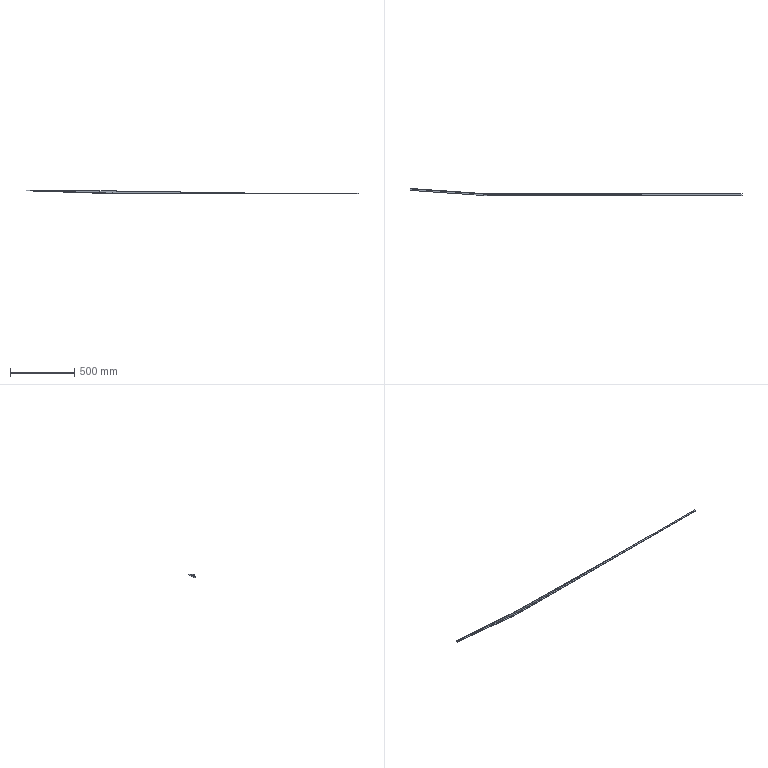Part | SolidWorks | features BaseBody 1 | 1 solid | 20 faces | box 2576 x 54.755 x 25.641 mm | volume 177267 mm3 | plane 20
STEP:
#1=CARTESIAN_POINT('',(-2.164,63.36,25.883));
#2=VERTEX_POINT('',#1);
#3=CARTESIAN_POINT('',(97.633,63.419,22.713));
#4=VERTEX_POINT('',#3);
#5=CARTESIAN_POINT('',(-2.164,63.36,25.883));
#6=CARTESIAN_POINT('',(31.101,63.38,24.826));
#7=CARTESIAN_POINT('',(64.367,63.4,23.77));
#8=CARTESIAN_POINT('',(97.633,63.419,22.713));
#9=B_SPLINE_CURVE_WITH_KNOTS('',3,(#5,#6,#7,#8),.UNSPECIFIED.,.F.,.F.,(4,4),(0.,1.),.UNSPECIFIED.);
#10=EDGE_CURVE('',#2,#4,#9,.T.);
#11=ORIENTED_EDGE('',*,*,#10,.F.);
#12=CARTESIAN_POINT('',(-2.388,60.16,25.827));
#13=VERTEX_POINT('',#12);
#14=CARTESIAN_POINT('',(-2.388,60.16,25.827));
#15=CARTESIAN_POINT('',(-2.313,61.227,25.845));
#16=CARTESIAN_POINT('',(-2.239,62.293,25.864));
#17=CARTESIAN_POINT('',(-2.164,63.36,25.883));
#18=B_SPLINE_CURVE_WITH_KNOTS('',3,(#14,#15,#16,#17),.UNSPECIFIED.,.F.,.F.,(4,4),(0.,1.),.UNSPECIFIED.);
#19=EDGE_CURVE('',#13,#2,#18,.T.);
#20=ORIENTED_EDGE('',*,*,#19,.F.);
#21=CARTESIAN_POINT('',(97.633,60.22,22.65));
#22=VERTEX_POINT('',#21);
#23=CARTESIAN_POINT('',(97.633,60.22,22.65));
#24=CARTESIAN_POINT('',(64.293,60.2,23.709));
#25=CARTESIAN_POINT('',(30.952,60.18,24.768));
#26=CARTESIAN_POINT('',(-2.388,60.16,25.827));
#27=B_SPLINE_CURVE_WITH_KNOTS('',3,(#23,#24,#25,#26),.UNSPECIFIED.,.F.,.F.,(4,4),(0.,1.),.UNSPECIFIED.);
#28=EDGE_CURVE('',#22,#13,#27,.T.);
#29=ORIENTED_EDGE('',*,*,#28,.F.);
#30=CARTESIAN_POINT('',(97.633,63.419,22.713));
#31=CARTESIAN_POINT('',(97.633,62.353,22.692));
#32=CARTESIAN_POINT('',(97.633,61.287,22.671));
#33=CARTESIAN_POINT('',(97.633,60.22,22.65));
#34=B_SPLINE_CURVE_WITH_KNOTS('',3,(#30,#31,#32,#33),.UNSPECIFIED.,.F.,.F.,(4,4),(0.,1.),.UNSPECIFIED.);
#35=EDGE_CURVE('',#4,#22,#34,.T.);
#36=ORIENTED_EDGE('',*,*,#35,.F.);
#37=EDGE_LOOP('',(#11,#20,#29,#36));
#38=FACE_OUTER_BOUND('',#37,.T.);
#39=CARTESIAN_POINT('',(98.233,60.141,22.63));
#40=DIRECTION('',(-0.03175,0.01966,-0.9993));
#41=DIRECTION('',(-0.9995,0.,0.03175));
#42=AXIS2_PLACEMENT_3D('',#39,#40,#41);
#43=PLANE('',#42);
#44=ADVANCED_FACE('',(#38),#43,.F.);
#45=ORIENTED_EDGE('',*,*,#35,.T.);
#46=CARTESIAN_POINT('',(1223.741,60.566,5.051));
#47=VERTEX_POINT('',#46);
#48=CARTESIAN_POINT('',(660.687,60.393,13.851));
#49=DIRECTION('',(-0.9999,-0.0003075,0.01563));
#50=VECTOR('',#49,1000.);
#51=LINE('',#48,#50);
#52=EDGE_CURVE('',#47,#22,#51,.T.);
#53=ORIENTED_EDGE('',*,*,#52,.F.);
#54=CARTESIAN_POINT('',(1223.741,63.766,5.114));
#55=VERTEX_POINT('',#54);
#56=CARTESIAN_POINT('',(1223.741,62.166,5.082));
#57=DIRECTION('',(0.,-0.9998,-0.01967));
#58=VECTOR('',#57,1000.);
#59=LINE('',#56,#58);
#60=EDGE_CURVE('',#55,#47,#59,.T.);
#61=ORIENTED_EDGE('',*,*,#60,.F.);
#62=CARTESIAN_POINT('',(660.687,63.593,13.914));
#63=DIRECTION('',(0.9999,0.0003075,-0.01563));
#64=VECTOR('',#63,1000.);
#65=LINE('',#62,#64);
#66=EDGE_CURVE('',#4,#55,#65,.T.);
#67=ORIENTED_EDGE('',*,*,#66,.F.);
#68=EDGE_LOOP('',(#45,#53,#61,#67));
#69=FACE_OUTER_BOUND('',#68,.T.);
#70=CARTESIAN_POINT('',(97.633,60.22,22.65));
#71=DIRECTION('',(-0.01563,0.01967,-0.9997));
#72=DIRECTION('',(0.,0.9998,0.01967));
#73=AXIS2_PLACEMENT_3D('',#70,#71,#72);
#74=PLANE('',#73);
#75=ADVANCED_FACE('',(#69),#74,.F.);
#76=CARTESIAN_POINT('',(-2.276,63.36,25.883));
#77=VERTEX_POINT('',#76);
#78=CARTESIAN_POINT('',(-2.164,63.36,25.883));
#79=CARTESIAN_POINT('',(-2.202,63.36,25.883));
#80=CARTESIAN_POINT('',(-2.239,63.36,25.883));
#81=CARTESIAN_POINT('',(-2.276,63.36,25.883));
#82=B_SPLINE_CURVE_WITH_KNOTS('',3,(#78,#79,#80,#81),.UNSPECIFIED.,.F.,.F.,(4,4),(0.,1.),.UNSPECIFIED.);
#83=EDGE_CURVE('',#2,#77,#82,.T.);
#84=ORIENTED_EDGE('',*,*,#83,.F.);
#85=ORIENTED_EDGE('',*,*,#10,.T.);
#86=CARTESIAN_POINT('',(97.303,63.829,1.914));
#87=VERTEX_POINT('',#86);
#88=CARTESIAN_POINT('',(97.303,63.829,1.914));
#89=CARTESIAN_POINT('',(97.413,63.692,8.847));
#90=CARTESIAN_POINT('',(97.523,63.556,15.78));
#91=CARTESIAN_POINT('',(97.633,63.419,22.713));
#92=B_SPLINE_CURVE_WITH_KNOTS('',3,(#88,#89,#90,#91),.UNSPECIFIED.,.F.,.F.,(4,4),(0.,1.),.UNSPECIFIED.);
#93=EDGE_CURVE('',#87,#4,#92,.T.);
#94=ORIENTED_EDGE('',*,*,#93,.F.);
#95=CARTESIAN_POINT('',(-2.937,63.769,5.098));
#96=VERTEX_POINT('',#95);
#97=CARTESIAN_POINT('',(-2.937,63.769,5.098));
#98=CARTESIAN_POINT('',(30.476,63.789,4.036));
#99=CARTESIAN_POINT('',(63.889,63.809,2.975));
#100=CARTESIAN_POINT('',(97.303,63.829,1.914));
#101=B_SPLINE_CURVE_WITH_KNOTS('',3,(#97,#98,#99,#100),.UNSPECIFIED.,.F.,.F.,(4,4),(0.,1.),.UNSPECIFIED.);
#102=EDGE_CURVE('',#96,#87,#101,.T.);
#103=ORIENTED_EDGE('',*,*,#102,.F.);
#104=CARTESIAN_POINT('',(-2.276,63.36,25.883));
#105=CARTESIAN_POINT('',(-2.496,63.496,18.954));
#106=CARTESIAN_POINT('',(-2.717,63.632,12.026));
#107=CARTESIAN_POINT('',(-2.937,63.769,5.098));
#108=B_SPLINE_CURVE_WITH_KNOTS('',3,(#104,#105,#106,#107),.UNSPECIFIED.,.F.,.F.,(4,4),(0.,1.),.UNSPECIFIED.);
#109=EDGE_CURVE('',#77,#96,#108,.T.);
#110=ORIENTED_EDGE('',*,*,#109,.F.);
#111=EDGE_LOOP('',(#84,#85,#94,#103,#110));
#112=FACE_OUTER_BOUND('',#111,.T.);
#113=CARTESIAN_POINT('',(-2.937,63.36,25.883));
#114=DIRECTION('',(-0.0000264,-0.9998,-0.01967));
#115=DIRECTION('',(0.,0.01967,-0.9998));
#116=AXIS2_PLACEMENT_3D('',#113,#114,#115);
#117=PLANE('',#116);
#118=ADVANCED_FACE('',(#112),#117,.F.);
#119=CARTESIAN_POINT('',(-575.334,100.207,27.204));
#120=VERTEX_POINT('',#119);
#121=CARTESIAN_POINT('',(-575.111,103.398,27.26));
#122=VERTEX_POINT('',#121);
#123=CARTESIAN_POINT('',(-575.334,100.207,27.204));
#124=CARTESIAN_POINT('',(-575.26,101.27,27.223));
#125=CARTESIAN_POINT('',(-575.185,102.334,27.241));
#126=CARTESIAN_POINT('',(-575.111,103.398,27.26));
#127=B_SPLINE_CURVE_WITH_KNOTS('',3,(#123,#124,#125,#126),.UNSPECIFIED.,.F.,.F.,(4,4),(0.,1.),.UNSPECIFIED.);
#128=EDGE_CURVE('',#120,#122,#127,.T.);
#129=ORIENTED_EDGE('',*,*,#128,.F.);
#130=CARTESIAN_POINT('',(-2.388,60.16,25.827));
#131=CARTESIAN_POINT('',(-193.37,73.509,26.286));
#132=CARTESIAN_POINT('',(-384.352,86.858,26.745));
#133=CARTESIAN_POINT('',(-575.334,100.207,27.204));
#134=B_SPLINE_CURVE_WITH_KNOTS('',3,(#130,#131,#132,#133),.UNSPECIFIED.,.F.,.F.,(4,4),(0.,1.),.UNSPECIFIED.);
#135=EDGE_CURVE('',#13,#120,#134,.T.);
#136=ORIENTED_EDGE('',*,*,#135,.F.);
#137=ORIENTED_EDGE('',*,*,#19,.T.);
#138=ORIENTED_EDGE('',*,*,#83,.T.);
#139=CARTESIAN_POINT('',(-575.111,103.398,27.26));
#140=CARTESIAN_POINT('',(-384.166,90.052,26.801));
#141=CARTESIAN_POINT('',(-193.221,76.706,26.342));
#142=CARTESIAN_POINT('',(-2.276,63.36,25.883));
#143=B_SPLINE_CURVE_WITH_KNOTS('',3,(#139,#140,#141,#142),.UNSPECIFIED.,.F.,.F.,(4,4),(0.,1.),.UNSPECIFIED.);
#144=EDGE_CURVE('',#122,#77,#143,.T.);
#145=ORIENTED_EDGE('',*,*,#144,.F.);
#146=EDGE_LOOP('',(#129,#136,#137,#138,#145));
#147=FACE_OUTER_BOUND('',#146,.T.);
#148=CARTESIAN_POINT('',(-575.334,60.148,26.502));
#149=DIRECTION('',(-0.001178,0.01753,-0.9998));
#150=DIRECTION('',(0.,0.9998,0.01753));
#151=AXIS2_PLACEMENT_3D('',#148,#149,#150);
#152=PLANE('',#151);
#153=ADVANCED_FACE('',(#147),#152,.F.);
#154=ORIENTED_EDGE('',*,*,#28,.T.);
#155=CARTESIAN_POINT('',(-2.947,60.506,8.236));
#156=VERTEX_POINT('',#155);
#157=CARTESIAN_POINT('',(-2.947,60.506,8.236));
#158=CARTESIAN_POINT('',(-2.761,60.391,14.1));
#159=CARTESIAN_POINT('',(-2.574,60.276,19.963));
#160=CARTESIAN_POINT('',(-2.388,60.16,25.827));
#161=B_SPLINE_CURVE_WITH_KNOTS('',3,(#157,#158,#159,#160),.UNSPECIFIED.,.F.,.F.,(4,4),(0.,1.),.UNSPECIFIED.);
#162=EDGE_CURVE('',#156,#13,#161,.T.);
#163=ORIENTED_EDGE('',*,*,#162,.F.);
#164=CARTESIAN_POINT('',(97.353,60.566,5.051));
#165=VERTEX_POINT('',#164);
#166=CARTESIAN_POINT('',(97.353,60.566,5.051));
#167=CARTESIAN_POINT('',(63.92,60.546,6.112));
#168=CARTESIAN_POINT('',(30.486,60.526,7.174));
#169=CARTESIAN_POINT('',(-2.947,60.506,8.236));
#170=B_SPLINE_CURVE_WITH_KNOTS('',3,(#166,#167,#168,#169),.UNSPECIFIED.,.F.,.F.,(4,4),(0.,1.),.UNSPECIFIED.);
#171=EDGE_CURVE('',#165,#156,#170,.T.);
#172=ORIENTED_EDGE('',*,*,#171,.F.);
#173=CARTESIAN_POINT('',(97.633,60.22,22.65));
#174=CARTESIAN_POINT('',(97.54,60.336,16.784));
#175=CARTESIAN_POINT('',(97.447,60.451,10.917));
#176=CARTESIAN_POINT('',(97.353,60.566,5.051));
#177=B_SPLINE_CURVE_WITH_KNOTS('',3,(#173,#174,#175,#176),.UNSPECIFIED.,.F.,.F.,(4,4),(0.,1.),.UNSPECIFIED.);
#178=EDGE_CURVE('',#22,#165,#177,.T.);
#179=ORIENTED_EDGE('',*,*,#178,.F.);
#180=EDGE_LOOP('',(#154,#163,#172,#179));
#181=FACE_OUTER_BOUND('',#180,.T.);
#182=CARTESIAN_POINT('',(-3.55,60.572,4.926));
#183=DIRECTION('',(0.0000264,0.9998,0.01967));
#184=DIRECTION('',(0.,-0.01967,0.9998));
#185=AXIS2_PLACEMENT_3D('',#182,#183,#184);
#186=PLANE('',#185);
#187=ADVANCED_FACE('',(#181),#186,.F.);
#188=ORIENTED_EDGE('',*,*,#93,.T.);
#189=ORIENTED_EDGE('',*,*,#66,.T.);
#190=CARTESIAN_POINT('',(2000.,63.766,5.114));
#191=VERTEX_POINT('',#190);
#192=CARTESIAN_POINT('',(1048.651,63.766,5.114));
#193=DIRECTION('',(1.,0.,0.));
#194=VECTOR('',#193,1000.);
#195=LINE('',#192,#194);
#196=EDGE_CURVE('',#55,#191,#195,.T.);
#197=ORIENTED_EDGE('',*,*,#196,.T.);
#198=CARTESIAN_POINT('',(2000.,63.829,1.914));
#199=VERTEX_POINT('',#198);
#200=CARTESIAN_POINT('',(2000.,63.624,12.314));
#201=DIRECTION('',(0.,0.01967,-0.9998));
#202=VECTOR('',#201,1000.);
#203=LINE('',#200,#202);
#204=EDGE_CURVE('',#191,#199,#203,.T.);
#205=ORIENTED_EDGE('',*,*,#204,.T.);
#206=CARTESIAN_POINT('',(1048.651,63.829,1.914));
#207=DIRECTION('',(-1.,0.,0.));
#208=VECTOR('',#207,1000.);
#209=LINE('',#206,#208);
#210=EDGE_CURVE('',#199,#87,#209,.T.);
#211=ORIENTED_EDGE('',*,*,#210,.T.);
#212=EDGE_LOOP('',(#188,#189,#197,#205,#211));
#213=FACE_OUTER_BOUND('',#212,.T.);
#214=CARTESIAN_POINT('',(97.303,63.829,1.914));
#215=DIRECTION('',(0.,0.9998,0.01967));
#216=DIRECTION('',(0.,-0.01967,0.9998));
#217=AXIS2_PLACEMENT_3D('',#214,#215,#216);
#218=PLANE('',#217);
#219=ADVANCED_FACE('',(#213),#218,.T.);
#220=ORIENTED_EDGE('',*,*,#178,.T.);
#221=CARTESIAN_POINT('',(660.547,60.566,5.051));
#222=DIRECTION('',(1.,0.,0.));
#223=VECTOR('',#222,1000.);
#224=LINE('',#221,#223);
#225=EDGE_CURVE('',#165,#47,#224,.T.);
#226=ORIENTED_EDGE('',*,*,#225,.T.);
#227=ORIENTED_EDGE('',*,*,#52,.T.);
#228=EDGE_LOOP('',(#220,#226,#227));
#229=FACE_OUTER_BOUND('',#228,.T.);
#230=CARTESIAN_POINT('',(90.595,60.218,22.756));
#231=DIRECTION('',(0.,-0.9998,-0.01967));
#232=DIRECTION('',(0.,0.01967,-0.9998));
#233=AXIS2_PLACEMENT_3D('',#230,#231,#232);
#234=PLANE('',#233);
#235=ADVANCED_FACE('',(#229),#234,.T.);
#236=ORIENTED_EDGE('',*,*,#225,.F.);
#237=CARTESIAN_POINT('',(97.353,48.766,4.818));
#238=VERTEX_POINT('',#237);
#239=CARTESIAN_POINT('',(97.353,60.566,5.051));
#240=CARTESIAN_POINT('',(97.353,56.633,4.973));
#241=CARTESIAN_POINT('',(97.353,52.7,4.896));
#242=CARTESIAN_POINT('',(97.353,48.766,4.818));
#243=B_SPLINE_CURVE_WITH_KNOTS('',3,(#239,#240,#241,#242),.UNSPECIFIED.,.F.,.F.,(4,4),(0.,1.),.UNSPECIFIED.);
#244=EDGE_CURVE('',#165,#238,#243,.T.);
#245=ORIENTED_EDGE('',*,*,#244,.T.);
#246=CARTESIAN_POINT('',(2000.,48.766,4.818));
#247=VERTEX_POINT('',#246);
#248=CARTESIAN_POINT('',(1048.677,48.766,4.818));
#249=DIRECTION('',(1.,0.,0.));
#250=VECTOR('',#249,1000.);
#251=LINE('',#248,#250);
#252=EDGE_CURVE('',#238,#247,#251,.T.);
#253=ORIENTED_EDGE('',*,*,#252,.T.);
#254=CARTESIAN_POINT('',(2000.,56.266,4.966));
#255=DIRECTION('',(0.,0.9998,0.01967));
#256=VECTOR('',#255,1000.);
#257=LINE('',#254,#256);
#258=EDGE_CURVE('',#247,#191,#257,.T.);
#259=ORIENTED_EDGE('',*,*,#258,.T.);
#260=ORIENTED_EDGE('',*,*,#196,.F.);
#261=ORIENTED_EDGE('',*,*,#60,.T.);
#262=EDGE_LOOP('',(#236,#245,#253,#259,#260,#261));
#263=FACE_OUTER_BOUND('',#262,.T.);
#264=CARTESIAN_POINT('',(97.353,63.766,5.114));
#265=DIRECTION('',(0.,-0.01967,0.9998));
#266=DIRECTION('',(0.,-0.9998,-0.01967));
#267=AXIS2_PLACEMENT_3D('',#264,#265,#266);
#268=PLANE('',#267);
#269=ADVANCED_FACE('',(#263),#268,.T.);
#270=CARTESIAN_POINT('',(-575.213,103.461,24.062));
#271=VERTEX_POINT('',#270);
#272=CARTESIAN_POINT('',(-2.937,63.769,5.098));
#273=CARTESIAN_POINT('',(-193.695,77.,11.419));
#274=CARTESIAN_POINT('',(-384.454,90.23,17.741));
#275=CARTESIAN_POINT('',(-575.213,103.461,24.062));
#276=B_SPLINE_CURVE_WITH_KNOTS('',3,(#272,#273,#274,#275),.UNSPECIFIED.,.F.,.F.,(4,4),(0.,1.),.UNSPECIFIED.);
#277=EDGE_CURVE('',#96,#271,#276,.T.);
#278=ORIENTED_EDGE('',*,*,#277,.T.);
#279=CARTESIAN_POINT('',(-575.213,103.461,24.062));
#280=CARTESIAN_POINT('',(-575.179,103.44,25.128));
#281=CARTESIAN_POINT('',(-575.145,103.419,26.194));
#282=CARTESIAN_POINT('',(-575.111,103.398,27.26));
#283=B_SPLINE_CURVE_WITH_KNOTS('',3,(#279,#280,#281,#282),.UNSPECIFIED.,.F.,.F.,(4,4),(0.,1.),.UNSPECIFIED.);
#284=EDGE_CURVE('',#271,#122,#283,.T.);
#285=ORIENTED_EDGE('',*,*,#284,.T.);
#286=ORIENTED_EDGE('',*,*,#144,.T.);
#287=ORIENTED_EDGE('',*,*,#109,.T.);
#288=EDGE_LOOP('',(#278,#285,#286,#287));
#289=FACE_OUTER_BOUND('',#288,.T.);
#290=CARTESIAN_POINT('',(1.187,63.483,4.965));
#291=DIRECTION('',(0.06976,0.9974,0.01741));
#292=DIRECTION('',(-0.9976,0.06977,0.));
#293=AXIS2_PLACEMENT_3D('',#290,#291,#292);
#294=PLANE('',#293);
#295=ADVANCED_FACE('',(#289),#294,.T.);
#296=CARTESIAN_POINT('',(-3.461,48.769,4.819));
#297=VERTEX_POINT('',#296);
#298=CARTESIAN_POINT('',(97.302,48.829,1.619));
#299=VERTEX_POINT('',#298);
#300=CARTESIAN_POINT('',(-3.461,48.769,4.819));
#301=CARTESIAN_POINT('',(30.127,48.789,3.752));
#302=CARTESIAN_POINT('',(63.715,48.809,2.686));
#303=CARTESIAN_POINT('',(97.302,48.829,1.619));
#304=B_SPLINE_CURVE_WITH_KNOTS('',3,(#300,#301,#302,#303),.UNSPECIFIED.,.F.,.F.,(4,4),(0.,1.),.UNSPECIFIED.);
#305=EDGE_CURVE('',#297,#299,#304,.T.);
#306=ORIENTED_EDGE('',*,*,#305,.F.);
#307=CARTESIAN_POINT('',(-2.937,63.769,5.098));
#308=CARTESIAN_POINT('',(-3.111,58.769,5.005));
#309=CARTESIAN_POINT('',(-3.286,53.769,4.912));
#310=CARTESIAN_POINT('',(-3.461,48.769,4.819));
#311=B_SPLINE_CURVE_WITH_KNOTS('',3,(#307,#308,#309,#310),.UNSPECIFIED.,.F.,.F.,(4,4),(0.,1.),.UNSPECIFIED.);
#312=EDGE_CURVE('',#96,#297,#311,.T.);
#313=ORIENTED_EDGE('',*,*,#312,.F.);
#314=ORIENTED_EDGE('',*,*,#102,.T.);
#315=CARTESIAN_POINT('',(97.302,48.829,1.619));
#316=CARTESIAN_POINT('',(97.302,53.829,1.717));
#317=CARTESIAN_POINT('',(97.303,58.829,1.816));
#318=CARTESIAN_POINT('',(97.303,63.829,1.914));
#319=B_SPLINE_CURVE_WITH_KNOTS('',3,(#315,#316,#317,#318),.UNSPECIFIED.,.F.,.F.,(4,4),(0.,1.),.UNSPECIFIED.);
#320=EDGE_CURVE('',#299,#87,#319,.T.);
#321=ORIENTED_EDGE('',*,*,#320,.F.);
#322=EDGE_LOOP('',(#306,#313,#314,#321));
#323=FACE_OUTER_BOUND('',#322,.T.);
#324=CARTESIAN_POINT('',(-4.065,48.679,4.837));
#325=DIRECTION('',(0.03175,-0.01966,0.9993));
#326=DIRECTION('',(0.9995,0.,-0.03175));
#327=AXIS2_PLACEMENT_3D('',#324,#325,#326);
#328=PLANE('',#327);
#329=ADVANCED_FACE('',(#323),#328,.F.);
#330=CARTESIAN_POINT('',(-576.259,88.498,23.801));
#331=VERTEX_POINT('',#330);
#332=CARTESIAN_POINT('',(-576.157,88.435,26.999));
#333=VERTEX_POINT('',#332);
#334=CARTESIAN_POINT('',(-576.259,88.498,23.801));
#335=CARTESIAN_POINT('',(-576.225,88.477,24.867));
#336=CARTESIAN_POINT('',(-576.191,88.456,25.933));
#337=CARTESIAN_POINT('',(-576.157,88.435,26.999));
#338=B_SPLINE_CURVE_WITH_KNOTS('',3,(#334,#335,#336,#337),.UNSPECIFIED.,.F.,.F.,(4,4),(0.,1.),.UNSPECIFIED.);
#339=EDGE_CURVE('',#331,#333,#338,.T.);
#340=ORIENTED_EDGE('',*,*,#339,.T.);
#341=CARTESIAN_POINT('',(-576.157,88.435,26.999));
#342=CARTESIAN_POINT('',(-575.883,92.359,27.067));
#343=CARTESIAN_POINT('',(-575.609,96.283,27.136));
#344=CARTESIAN_POINT('',(-575.334,100.207,27.204));
#345=B_SPLINE_CURVE_WITH_KNOTS('',3,(#341,#342,#343,#344),.UNSPECIFIED.,.F.,.F.,(4,4),(0.,1.),.UNSPECIFIED.);
#346=EDGE_CURVE('',#333,#120,#345,.T.);
#347=ORIENTED_EDGE('',*,*,#346,.T.);
#348=ORIENTED_EDGE('',*,*,#128,.T.);
#349=ORIENTED_EDGE('',*,*,#284,.F.);
#350=CARTESIAN_POINT('',(-575.213,103.461,24.062));
#351=CARTESIAN_POINT('',(-575.561,98.473,23.975));
#352=CARTESIAN_POINT('',(-575.91,93.486,23.888));
#353=CARTESIAN_POINT('',(-576.259,88.498,23.801));
#354=B_SPLINE_CURVE_WITH_KNOTS('',3,(#350,#351,#352,#353),.UNSPECIFIED.,.F.,.F.,(4,4),(0.,1.),.UNSPECIFIED.);
#355=EDGE_CURVE('',#271,#331,#354,.T.);
#356=ORIENTED_EDGE('',*,*,#355,.T.);
#357=EDGE_LOOP('',(#340,#347,#348,#349,#356));
#358=FACE_OUTER_BOUND('',#357,.T.);
#359=CARTESIAN_POINT('',(-575.221,103.462,23.801));
#360=DIRECTION('',(-0.9971,0.06916,0.03304));
#361=DIRECTION('',(-0.06919,-0.9976,0.));
#362=AXIS2_PLACEMENT_3D('',#359,#360,#361);
#363=PLANE('',#362);
#364=ADVANCED_FACE('',(#358),#363,.T.);
#365=CARTESIAN_POINT('',(-575.334,100.207,27.204));
#366=CARTESIAN_POINT('',(-384.538,86.973,20.881));
#367=CARTESIAN_POINT('',(-193.743,73.74,14.559));
#368=CARTESIAN_POINT('',(-2.947,60.506,8.236));
#369=B_SPLINE_CURVE_WITH_KNOTS('',3,(#365,#366,#367,#368),.UNSPECIFIED.,.F.,.F.,(4,4),(0.,1.),.UNSPECIFIED.);
#370=EDGE_CURVE('',#120,#156,#369,.T.);
#371=ORIENTED_EDGE('',*,*,#370,.T.);
#372=ORIENTED_EDGE('',*,*,#162,.T.);
#373=ORIENTED_EDGE('',*,*,#135,.T.);
#374=EDGE_LOOP('',(#371,#372,#373));
#375=FACE_OUTER_BOUND('',#374,.T.);
#376=CARTESIAN_POINT('',(-578.749,100.778,8.122));
#377=DIRECTION('',(-0.06976,-0.9974,-0.01741));
#378=DIRECTION('',(0.9976,-0.06977,0.));
#379=AXIS2_PLACEMENT_3D('',#376,#377,#378);
#380=PLANE('',#379);
#381=ADVANCED_FACE('',(#375),#380,.T.);
#382=ORIENTED_EDGE('',*,*,#171,.T.);
#383=CARTESIAN_POINT('',(-3.359,48.706,8.017));
#384=VERTEX_POINT('',#383);
#385=CARTESIAN_POINT('',(-3.359,48.706,8.017));
#386=CARTESIAN_POINT('',(-3.222,52.64,8.09));
#387=CARTESIAN_POINT('',(-3.084,56.573,8.163));
#388=CARTESIAN_POINT('',(-2.947,60.506,8.236));
#389=B_SPLINE_CURVE_WITH_KNOTS('',3,(#385,#386,#387,#388),.UNSPECIFIED.,.F.,.F.,(4,4),(0.,1.),.UNSPECIFIED.);
#390=EDGE_CURVE('',#384,#156,#389,.T.);
#391=ORIENTED_EDGE('',*,*,#390,.F.);
#392=CARTESIAN_POINT('',(97.353,48.766,4.818));
#393=CARTESIAN_POINT('',(63.782,48.746,5.885));
#394=CARTESIAN_POINT('',(30.212,48.726,6.951));
#395=CARTESIAN_POINT('',(-3.359,48.706,8.017));
#396=B_SPLINE_CURVE_WITH_KNOTS('',3,(#392,#393,#394,#395),.UNSPECIFIED.,.F.,.F.,(4,4),(0.,1.),.UNSPECIFIED.);
#397=EDGE_CURVE('',#238,#384,#396,.T.);
#398=ORIENTED_EDGE('',*,*,#397,.F.);
#399=ORIENTED_EDGE('',*,*,#244,.F.);
#400=EDGE_LOOP('',(#382,#391,#398,#399));
#401=FACE_OUTER_BOUND('',#400,.T.);
#402=CARTESIAN_POINT('',(97.957,48.635,4.797));
#403=DIRECTION('',(-0.03175,0.01966,-0.9993));
#404=DIRECTION('',(-0.9995,0.,0.03175));
#405=AXIS2_PLACEMENT_3D('',#402,#403,#404);
#406=PLANE('',#405);
#407=ADVANCED_FACE('',(#401),#406,.F.);
#408=CARTESIAN_POINT('',(2000.,48.829,1.619));
#409=VERTEX_POINT('',#408);
#410=CARTESIAN_POINT('',(1042.943,48.829,1.619));
#411=DIRECTION('',(-1.,0.,0.));
#412=VECTOR('',#411,1000.);
#413=LINE('',#410,#412);
#414=EDGE_CURVE('',#409,#299,#413,.T.);
#415=ORIENTED_EDGE('',*,*,#414,.T.);
#416=ORIENTED_EDGE('',*,*,#320,.T.);
#417=ORIENTED_EDGE('',*,*,#210,.F.);
#418=CARTESIAN_POINT('',(2000.,56.329,1.767));
#419=DIRECTION('',(0.,-0.9998,-0.01967));
#420=VECTOR('',#419,1000.);
#421=LINE('',#418,#420);
#422=EDGE_CURVE('',#199,#409,#421,.T.);
#423=ORIENTED_EDGE('',*,*,#422,.T.);
#424=EDGE_LOOP('',(#415,#416,#417,#423));
#425=FACE_OUTER_BOUND('',#424,.T.);
#426=CARTESIAN_POINT('',(85.886,48.829,1.619));
#427=DIRECTION('',(0.,0.01967,-0.9998));
#428=DIRECTION('',(0.,0.9998,0.01967));
#429=AXIS2_PLACEMENT_3D('',#426,#427,#428);
#430=PLANE('',#429);
#431=ADVANCED_FACE('',(#425),#430,.T.);
#432=CARTESIAN_POINT('',(2000.,48.766,4.818));
#433=CARTESIAN_POINT('',(2000.,48.787,3.752));
#434=CARTESIAN_POINT('',(2000.,48.808,2.686));
#435=CARTESIAN_POINT('',(2000.,48.829,1.619));
#436=B_SPLINE_CURVE_WITH_KNOTS('',3,(#432,#433,#434,#435),.UNSPECIFIED.,.F.,.F.,(4,4),(0.,1.),.UNSPECIFIED.);
#437=EDGE_CURVE('',#247,#409,#436,.T.);
#438=ORIENTED_EDGE('',*,*,#437,.T.);
#439=ORIENTED_EDGE('',*,*,#422,.F.);
#440=ORIENTED_EDGE('',*,*,#204,.F.);
#441=ORIENTED_EDGE('',*,*,#258,.F.);
#442=EDGE_LOOP('',(#438,#439,#440,#441));
#443=FACE_OUTER_BOUND('',#442,.T.);
#444=CARTESIAN_POINT('',(2000.,48.676,5.135));
#445=DIRECTION('',(1.,0.,0.));
#446=DIRECTION('',(0.,0.,-1.));
#447=AXIS2_PLACEMENT_3D('',#444,#445,#446);
#448=PLANE('',#447);
#449=ADVANCED_FACE('',(#443),#448,.T.);
#450=ORIENTED_EDGE('',*,*,#252,.F.);
#451=CARTESIAN_POINT('',(97.353,48.766,4.818));
#452=CARTESIAN_POINT('',(97.336,48.787,3.752));
#453=CARTESIAN_POINT('',(97.319,48.808,2.686));
#454=CARTESIAN_POINT('',(97.302,48.829,1.619));
#455=B_SPLINE_CURVE_WITH_KNOTS('',3,(#451,#452,#453,#454),.UNSPECIFIED.,.F.,.F.,(4,4),(0.,1.),.UNSPECIFIED.);
#456=EDGE_CURVE('',#238,#299,#455,.T.);
#457=ORIENTED_EDGE('',*,*,#456,.T.);
#458=ORIENTED_EDGE('',*,*,#414,.F.);
#459=ORIENTED_EDGE('',*,*,#437,.F.);
#460=EDGE_LOOP('',(#450,#457,#458,#459));
#461=FACE_OUTER_BOUND('',#460,.T.);
#462=CARTESIAN_POINT('',(85.886,48.766,4.818));
#463=DIRECTION('',(0.,-0.9998,-0.01967));
#464=DIRECTION('',(0.,0.01967,-0.9998));
#465=AXIS2_PLACEMENT_3D('',#462,#463,#464);
#466=PLANE('',#465);
#467=ADVANCED_FACE('',(#461),#466,.T.);
#468=CARTESIAN_POINT('',(-3.461,48.769,4.819));
#469=CARTESIAN_POINT('',(-194.394,62.012,11.146));
#470=CARTESIAN_POINT('',(-385.326,75.255,17.474));
#471=CARTESIAN_POINT('',(-576.259,88.498,23.801));
#472=B_SPLINE_CURVE_WITH_KNOTS('',3,(#468,#469,#470,#471),.UNSPECIFIED.,.F.,.F.,(4,4),(0.,1.),.UNSPECIFIED.);
#473=EDGE_CURVE('',#297,#331,#472,.T.);
#474=ORIENTED_EDGE('',*,*,#473,.T.);
#475=ORIENTED_EDGE('',*,*,#355,.F.);
#476=ORIENTED_EDGE('',*,*,#277,.F.);
#477=ORIENTED_EDGE('',*,*,#312,.T.);
#478=EDGE_LOOP('',(#474,#475,#476,#477));
#479=FACE_OUTER_BOUND('',#478,.T.);
#480=CARTESIAN_POINT('',(0.4937,48.441,4.687));
#481=DIRECTION('',(-0.03175,0.01966,-0.9993));
#482=DIRECTION('',(-0.9995,0.,0.03176));
#483=AXIS2_PLACEMENT_3D('',#480,#481,#482);
#484=PLANE('',#483);
#485=ADVANCED_FACE('',(#479),#484,.T.);
#486=ORIENTED_EDGE('',*,*,#397,.T.);
#487=CARTESIAN_POINT('',(-3.461,48.769,4.819));
#488=CARTESIAN_POINT('',(-3.427,48.748,5.885));
#489=CARTESIAN_POINT('',(-3.393,48.727,6.951));
#490=CARTESIAN_POINT('',(-3.359,48.706,8.017));
#491=B_SPLINE_CURVE_WITH_KNOTS('',3,(#487,#488,#489,#490),.UNSPECIFIED.,.F.,.F.,(4,4),(0.,1.),.UNSPECIFIED.);
#492=EDGE_CURVE('',#297,#384,#491,.T.);
#493=ORIENTED_EDGE('',*,*,#492,.F.);
#494=ORIENTED_EDGE('',*,*,#305,.T.);
#495=ORIENTED_EDGE('',*,*,#456,.F.);
#496=EDGE_LOOP('',(#486,#493,#494,#495));
#497=FACE_OUTER_BOUND('',#496,.T.);
#498=CARTESIAN_POINT('',(-4.066,48.833,1.581));
#499=DIRECTION('',(0.0000264,0.9998,0.01967));
#500=DIRECTION('',(0.,-0.01967,0.9998));
#501=AXIS2_PLACEMENT_3D('',#498,#499,#500);
#502=PLANE('',#501);
#503=ADVANCED_FACE('',(#497),#502,.F.);
#504=ORIENTED_EDGE('',*,*,#370,.F.);
#505=ORIENTED_EDGE('',*,*,#346,.F.);
#506=CARTESIAN_POINT('',(-576.157,88.435,26.999));
#507=CARTESIAN_POINT('',(-385.225,75.192,20.671));
#508=CARTESIAN_POINT('',(-194.292,61.949,14.344));
#509=CARTESIAN_POINT('',(-3.359,48.706,8.017));
#510=B_SPLINE_CURVE_WITH_KNOTS('',3,(#506,#507,#508,#509),.UNSPECIFIED.,.F.,.F.,(4,4),(0.,1.),.UNSPECIFIED.);
#511=EDGE_CURVE('',#333,#384,#510,.T.);
#512=ORIENTED_EDGE('',*,*,#511,.T.);
#513=ORIENTED_EDGE('',*,*,#390,.T.);
#514=EDGE_LOOP('',(#504,#505,#512,#513));
#515=FACE_OUTER_BOUND('',#514,.T.);
#516=CARTESIAN_POINT('',(-579.622,48.397,26.321));
#517=DIRECTION('',(0.03175,-0.01966,0.9993));
#518=DIRECTION('',(0.9995,0.,-0.03176));
#519=AXIS2_PLACEMENT_3D('',#516,#517,#518);
#520=PLANE('',#519);
#521=ADVANCED_FACE('',(#515),#520,.T.);
#522=ORIENTED_EDGE('',*,*,#511,.F.);
#523=ORIENTED_EDGE('',*,*,#339,.F.);
#524=ORIENTED_EDGE('',*,*,#473,.F.);
#525=ORIENTED_EDGE('',*,*,#492,.T.);
#526=EDGE_LOOP('',(#522,#523,#524,#525));
#527=FACE_OUTER_BOUND('',#526,.T.);
#528=CARTESIAN_POINT('',(-579.673,89.07,4.686));
#529=DIRECTION('',(-0.06976,-0.9974,-0.01741));
#530=DIRECTION('',(0.9976,-0.06977,0.));
#531=AXIS2_PLACEMENT_3D('',#528,#529,#530);
#532=PLANE('',#531);
#533=ADVANCED_FACE('',(#527),#532,.T.);
#534=CLOSED_SHELL('',(#44,#75,#118,#153,#187,#219,#235,#269,#295,#329,#364,#381,#407,#431,#449,#467,#485,#503,#521,#533));
#535=MANIFOLD_SOLID_BREP('',#534);
#536=CARTESIAN_POINT('',(0.,0.,0.));
#537=DIRECTION('',(0.,0.,1.));
#538=DIRECTION('',(1.,0.,0.));
#539=AXIS2_PLACEMENT_3D('',#536,#537,#538);
#540=(LENGTH_UNIT()NAMED_UNIT(*)SI_UNIT(.MILLI.,.METRE.));
#541=UNCERTAINTY_MEASURE_WITH_UNIT(LENGTH_MEASURE(0.00001),#540,'','');
#542=(NAMED_UNIT(*)PLANE_ANGLE_UNIT()SI_UNIT($,.RADIAN.));
#543=(NAMED_UNIT(*)SI_UNIT($,.STERADIAN.)SOLID_ANGLE_UNIT());
#544=(GEOMETRIC_REPRESENTATION_CONTEXT(3)GLOBAL_UNCERTAINTY_ASSIGNED_CONTEXT((#541))GLOBAL_UNIT_ASSIGNED_CONTEXT((#540,#542,#543))REPRESENTATION_CONTEXT('',''));
#545=ADVANCED_BREP_SHAPE_REPRESENTATION('',(#535,#539),#544);